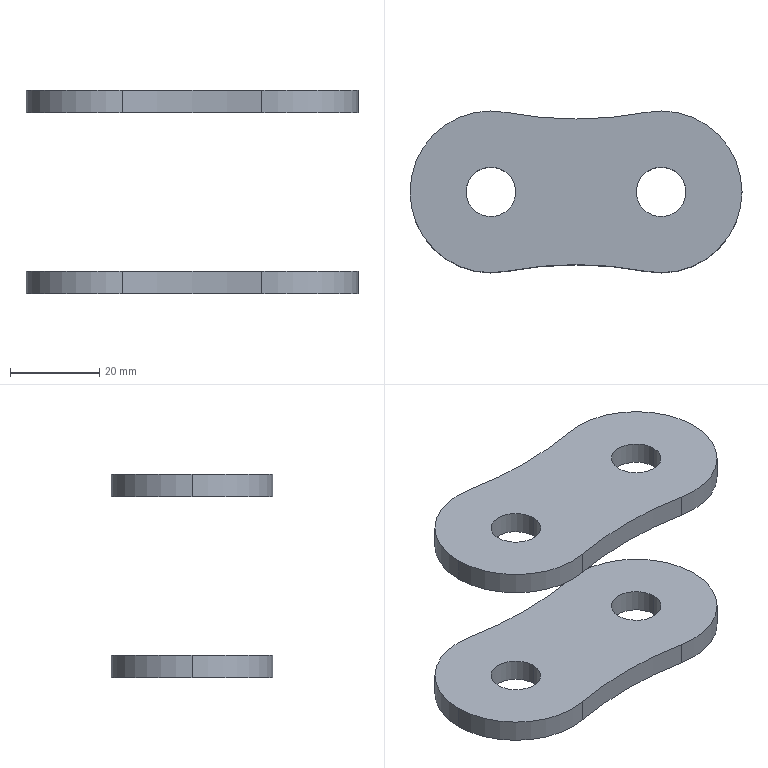Part | SolidWorks | features BaseBody 2 | 2 solids | 22 faces | box 74.3 x 36.2 x 45.44 mm | volume 21265 mm3 | cylinder 18 | plane 4 | commonest cylinder face diameters 11.11 x8 36.2 x6 166.109 x4
STEP:
#1=CARTESIAN_POINT('',(-24.605,0.,22.72));
#2=VERTEX_POINT('',#1);
#3=CARTESIAN_POINT('',(-13.495,0.,22.72));
#4=VERTEX_POINT('',#3);
#5=CARTESIAN_POINT('',(-19.05,0.,22.72));
#6=DIRECTION('',(0.,0.,1.));
#7=DIRECTION('',(1.,0.,0.));
#8=AXIS2_PLACEMENT_3D('',#5,#6,#7);
#9=CIRCLE('',#8,5.555);
#10=EDGE_CURVE('',#2,#4,#9,.T.);
#11=ORIENTED_EDGE('',*,*,#10,.T.);
#12=CARTESIAN_POINT('',(-13.495,0.,17.73));
#13=VERTEX_POINT('',#12);
#14=CARTESIAN_POINT('',(-13.495,0.,22.72));
#15=DIRECTION('',(0.,0.,-1.));
#16=VECTOR('',#15,1000.);
#17=LINE('',#14,#16);
#18=EDGE_CURVE('',#4,#13,#17,.T.);
#19=ORIENTED_EDGE('',*,*,#18,.T.);
#20=CARTESIAN_POINT('',(-24.605,0.,17.73));
#21=VERTEX_POINT('',#20);
#22=CARTESIAN_POINT('',(-19.05,0.,17.73));
#23=DIRECTION('',(0.,0.,1.));
#24=DIRECTION('',(1.,0.,0.));
#25=AXIS2_PLACEMENT_3D('',#22,#23,#24);
#26=CIRCLE('',#25,5.555);
#27=EDGE_CURVE('',#21,#13,#26,.T.);
#28=ORIENTED_EDGE('',*,*,#27,.F.);
#29=CARTESIAN_POINT('',(-24.605,0.,22.72));
#30=DIRECTION('',(0.,0.,-1.));
#31=VECTOR('',#30,1000.);
#32=LINE('',#29,#31);
#33=EDGE_CURVE('',#2,#21,#32,.T.);
#34=ORIENTED_EDGE('',*,*,#33,.F.);
#35=EDGE_LOOP('',(#11,#19,#28,#34));
#36=FACE_OUTER_BOUND('',#35,.T.);
#37=CARTESIAN_POINT('',(-19.05,0.,22.72));
#38=DIRECTION('',(0.,0.,-1.));
#39=DIRECTION('',(-1.,0.,0.));
#40=AXIS2_PLACEMENT_3D('',#37,#38,#39);
#41=CYLINDRICAL_SURFACE('',#40,5.555);
#42=ADVANCED_FACE('',(#36),#41,.F.);
#43=CARTESIAN_POINT('',(13.495,0.,22.72));
#44=VERTEX_POINT('',#43);
#45=CARTESIAN_POINT('',(24.605,0.,22.72));
#46=VERTEX_POINT('',#45);
#47=CARTESIAN_POINT('',(19.05,0.,22.72));
#48=DIRECTION('',(0.,0.,1.));
#49=DIRECTION('',(1.,0.,0.));
#50=AXIS2_PLACEMENT_3D('',#47,#48,#49);
#51=CIRCLE('',#50,5.555);
#52=EDGE_CURVE('',#44,#46,#51,.T.);
#53=ORIENTED_EDGE('',*,*,#52,.T.);
#54=CARTESIAN_POINT('',(24.605,0.,17.73));
#55=VERTEX_POINT('',#54);
#56=CARTESIAN_POINT('',(24.605,0.,22.72));
#57=DIRECTION('',(0.,0.,-1.));
#58=VECTOR('',#57,1000.);
#59=LINE('',#56,#58);
#60=EDGE_CURVE('',#46,#55,#59,.T.);
#61=ORIENTED_EDGE('',*,*,#60,.T.);
#62=CARTESIAN_POINT('',(13.495,0.,17.73));
#63=VERTEX_POINT('',#62);
#64=CARTESIAN_POINT('',(19.05,0.,17.73));
#65=DIRECTION('',(0.,0.,1.));
#66=DIRECTION('',(1.,0.,0.));
#67=AXIS2_PLACEMENT_3D('',#64,#65,#66);
#68=CIRCLE('',#67,5.555);
#69=EDGE_CURVE('',#63,#55,#68,.T.);
#70=ORIENTED_EDGE('',*,*,#69,.F.);
#71=CARTESIAN_POINT('',(13.495,0.,22.72));
#72=DIRECTION('',(0.,0.,-1.));
#73=VECTOR('',#72,1000.);
#74=LINE('',#71,#73);
#75=EDGE_CURVE('',#44,#63,#74,.T.);
#76=ORIENTED_EDGE('',*,*,#75,.F.);
#77=EDGE_LOOP('',(#53,#61,#70,#76));
#78=FACE_OUTER_BOUND('',#77,.T.);
#79=CARTESIAN_POINT('',(19.05,0.,22.72));
#80=DIRECTION('',(0.,0.,-1.));
#81=DIRECTION('',(-1.,0.,0.));
#82=AXIS2_PLACEMENT_3D('',#79,#80,#81);
#83=CYLINDRICAL_SURFACE('',#82,5.555);
#84=ADVANCED_FACE('',(#78),#83,.F.);
#85=CARTESIAN_POINT('',(-37.15,0.,22.72));
#86=VERTEX_POINT('',#85);
#87=CARTESIAN_POINT('',(-15.641,-17.776,22.72));
#88=VERTEX_POINT('',#87);
#89=CARTESIAN_POINT('',(-19.05,0.,22.72));
#90=DIRECTION('',(0.,0.,1.));
#91=DIRECTION('',(1.,0.,0.));
#92=AXIS2_PLACEMENT_3D('',#89,#90,#91);
#93=CIRCLE('',#92,18.1);
#94=EDGE_CURVE('',#86,#88,#93,.T.);
#95=ORIENTED_EDGE('',*,*,#94,.F.);
#96=CARTESIAN_POINT('',(-37.15,0.,17.73));
#97=VERTEX_POINT('',#96);
#98=CARTESIAN_POINT('',(-37.15,0.,22.72));
#99=DIRECTION('',(0.,0.,-1.));
#100=VECTOR('',#99,1000.);
#101=LINE('',#98,#100);
#102=EDGE_CURVE('',#86,#97,#101,.T.);
#103=ORIENTED_EDGE('',*,*,#102,.T.);
#104=CARTESIAN_POINT('',(-15.641,-17.776,17.73));
#105=VERTEX_POINT('',#104);
#106=CARTESIAN_POINT('',(-19.05,0.,17.73));
#107=DIRECTION('',(0.,0.,1.));
#108=DIRECTION('',(1.,0.,0.));
#109=AXIS2_PLACEMENT_3D('',#106,#107,#108);
#110=CIRCLE('',#109,18.1);
#111=EDGE_CURVE('',#97,#105,#110,.T.);
#112=ORIENTED_EDGE('',*,*,#111,.T.);
#113=CARTESIAN_POINT('',(-15.641,-17.776,22.72));
#114=DIRECTION('',(0.,0.,-1.));
#115=VECTOR('',#114,1000.);
#116=LINE('',#113,#115);
#117=EDGE_CURVE('',#88,#105,#116,.T.);
#118=ORIENTED_EDGE('',*,*,#117,.F.);
#119=EDGE_LOOP('',(#95,#103,#112,#118));
#120=FACE_OUTER_BOUND('',#119,.T.);
#121=CARTESIAN_POINT('',(-19.05,0.,22.72));
#122=DIRECTION('',(0.,0.,-1.));
#123=DIRECTION('',(-1.,0.,0.));
#124=AXIS2_PLACEMENT_3D('',#121,#122,#123);
#125=CYLINDRICAL_SURFACE('',#124,18.1);
#126=ADVANCED_FACE('',(#120),#125,.T.);
#127=ORIENTED_EDGE('',*,*,#52,.F.);
#128=CARTESIAN_POINT('',(19.05,0.,22.72));
#129=DIRECTION('',(0.,0.,1.));
#130=DIRECTION('',(1.,0.,0.));
#131=AXIS2_PLACEMENT_3D('',#128,#129,#130);
#132=CIRCLE('',#131,5.555);
#133=EDGE_CURVE('',#46,#44,#132,.T.);
#134=ORIENTED_EDGE('',*,*,#133,.F.);
#135=EDGE_LOOP('',(#127,#134));
#136=FACE_BOUND('',#135,.T.);
#137=CARTESIAN_POINT('',(15.641,-17.776,22.72));
#138=VERTEX_POINT('',#137);
#139=CARTESIAN_POINT('',(0.,-99.344,22.72));
#140=DIRECTION('',(0.,0.,-1.));
#141=DIRECTION('',(1.,0.,0.));
#142=AXIS2_PLACEMENT_3D('',#139,#140,#141);
#143=CIRCLE('',#142,83.054);
#144=EDGE_CURVE('',#88,#138,#143,.T.);
#145=ORIENTED_EDGE('',*,*,#144,.T.);
#146=CARTESIAN_POINT('',(15.641,17.776,22.72));
#147=VERTEX_POINT('',#146);
#148=CARTESIAN_POINT('',(19.05,0.,22.72));
#149=DIRECTION('',(0.,0.,1.));
#150=DIRECTION('',(1.,0.,0.));
#151=AXIS2_PLACEMENT_3D('',#148,#149,#150);
#152=CIRCLE('',#151,18.1);
#153=EDGE_CURVE('',#138,#147,#152,.T.);
#154=ORIENTED_EDGE('',*,*,#153,.T.);
#155=CARTESIAN_POINT('',(-15.641,17.776,22.72));
#156=VERTEX_POINT('',#155);
#157=CARTESIAN_POINT('',(0.,99.344,22.72));
#158=DIRECTION('',(0.,0.,-1.));
#159=DIRECTION('',(-1.,0.,0.));
#160=AXIS2_PLACEMENT_3D('',#157,#158,#159);
#161=CIRCLE('',#160,83.054);
#162=EDGE_CURVE('',#147,#156,#161,.T.);
#163=ORIENTED_EDGE('',*,*,#162,.T.);
#164=CARTESIAN_POINT('',(-19.05,0.,22.72));
#165=DIRECTION('',(0.,0.,1.));
#166=DIRECTION('',(1.,0.,0.));
#167=AXIS2_PLACEMENT_3D('',#164,#165,#166);
#168=CIRCLE('',#167,18.1);
#169=EDGE_CURVE('',#156,#86,#168,.T.);
#170=ORIENTED_EDGE('',*,*,#169,.T.);
#171=ORIENTED_EDGE('',*,*,#94,.T.);
#172=EDGE_LOOP('',(#145,#154,#163,#170,#171));
#173=FACE_OUTER_BOUND('',#172,.T.);
#174=ORIENTED_EDGE('',*,*,#10,.F.);
#175=CARTESIAN_POINT('',(-19.05,0.,22.72));
#176=DIRECTION('',(0.,0.,1.));
#177=DIRECTION('',(1.,0.,0.));
#178=AXIS2_PLACEMENT_3D('',#175,#176,#177);
#179=CIRCLE('',#178,5.555);
#180=EDGE_CURVE('',#4,#2,#179,.T.);
#181=ORIENTED_EDGE('',*,*,#180,.F.);
#182=EDGE_LOOP('',(#174,#181));
#183=FACE_BOUND('',#182,.T.);
#184=CARTESIAN_POINT('',(-9.525,-49.672,22.72));
#185=DIRECTION('',(0.,0.,1.));
#186=DIRECTION('',(1.,0.,0.));
#187=AXIS2_PLACEMENT_3D('',#184,#185,#186);
#188=PLANE('',#187);
#189=ADVANCED_FACE('',(#136,#173,#183),#188,.T.);
#190=CARTESIAN_POINT('',(15.641,-17.776,17.73));
#191=VERTEX_POINT('',#190);
#192=CARTESIAN_POINT('',(0.,-99.344,17.73));
#193=DIRECTION('',(0.,0.,-1.));
#194=DIRECTION('',(1.,0.,0.));
#195=AXIS2_PLACEMENT_3D('',#192,#193,#194);
#196=CIRCLE('',#195,83.054);
#197=EDGE_CURVE('',#105,#191,#196,.T.);
#198=ORIENTED_EDGE('',*,*,#197,.F.);
#199=ORIENTED_EDGE('',*,*,#111,.F.);
#200=CARTESIAN_POINT('',(-15.641,17.776,17.73));
#201=VERTEX_POINT('',#200);
#202=CARTESIAN_POINT('',(-19.05,0.,17.73));
#203=DIRECTION('',(0.,0.,1.));
#204=DIRECTION('',(1.,0.,0.));
#205=AXIS2_PLACEMENT_3D('',#202,#203,#204);
#206=CIRCLE('',#205,18.1);
#207=EDGE_CURVE('',#201,#97,#206,.T.);
#208=ORIENTED_EDGE('',*,*,#207,.F.);
#209=CARTESIAN_POINT('',(15.641,17.776,17.73));
#210=VERTEX_POINT('',#209);
#211=CARTESIAN_POINT('',(0.,99.344,17.73));
#212=DIRECTION('',(0.,0.,-1.));
#213=DIRECTION('',(-1.,0.,0.));
#214=AXIS2_PLACEMENT_3D('',#211,#212,#213);
#215=CIRCLE('',#214,83.054);
#216=EDGE_CURVE('',#210,#201,#215,.T.);
#217=ORIENTED_EDGE('',*,*,#216,.F.);
#218=CARTESIAN_POINT('',(19.05,0.,17.73));
#219=DIRECTION('',(0.,0.,1.));
#220=DIRECTION('',(1.,0.,0.));
#221=AXIS2_PLACEMENT_3D('',#218,#219,#220);
#222=CIRCLE('',#221,18.1);
#223=EDGE_CURVE('',#191,#210,#222,.T.);
#224=ORIENTED_EDGE('',*,*,#223,.F.);
#225=EDGE_LOOP('',(#198,#199,#208,#217,#224));
#226=FACE_OUTER_BOUND('',#225,.T.);
#227=ORIENTED_EDGE('',*,*,#69,.T.);
#228=CARTESIAN_POINT('',(19.05,0.,17.73));
#229=DIRECTION('',(0.,0.,1.));
#230=DIRECTION('',(1.,0.,0.));
#231=AXIS2_PLACEMENT_3D('',#228,#229,#230);
#232=CIRCLE('',#231,5.555);
#233=EDGE_CURVE('',#55,#63,#232,.T.);
#234=ORIENTED_EDGE('',*,*,#233,.T.);
#235=EDGE_LOOP('',(#227,#234));
#236=FACE_BOUND('',#235,.T.);
#237=ORIENTED_EDGE('',*,*,#27,.T.);
#238=CARTESIAN_POINT('',(-19.05,0.,17.73));
#239=DIRECTION('',(0.,0.,1.));
#240=DIRECTION('',(1.,0.,0.));
#241=AXIS2_PLACEMENT_3D('',#238,#239,#240);
#242=CIRCLE('',#241,5.555);
#243=EDGE_CURVE('',#13,#21,#242,.T.);
#244=ORIENTED_EDGE('',*,*,#243,.T.);
#245=EDGE_LOOP('',(#237,#244));
#246=FACE_BOUND('',#245,.T.);
#247=CARTESIAN_POINT('',(-9.525,-49.672,17.73));
#248=DIRECTION('',(0.,0.,1.));
#249=DIRECTION('',(1.,0.,0.));
#250=AXIS2_PLACEMENT_3D('',#247,#248,#249);
#251=PLANE('',#250);
#252=ADVANCED_FACE('',(#226,#236,#246),#251,.F.);
#253=ORIENTED_EDGE('',*,*,#197,.T.);
#254=CARTESIAN_POINT('',(15.641,-17.776,22.72));
#255=DIRECTION('',(0.,0.,-1.));
#256=VECTOR('',#255,1000.);
#257=LINE('',#254,#256);
#258=EDGE_CURVE('',#138,#191,#257,.T.);
#259=ORIENTED_EDGE('',*,*,#258,.F.);
#260=ORIENTED_EDGE('',*,*,#144,.F.);
#261=ORIENTED_EDGE('',*,*,#117,.T.);
#262=EDGE_LOOP('',(#253,#259,#260,#261));
#263=FACE_OUTER_BOUND('',#262,.T.);
#264=CARTESIAN_POINT('',(0.,-99.344,22.72));
#265=DIRECTION('',(0.,0.,-1.));
#266=DIRECTION('',(-1.,0.,0.));
#267=AXIS2_PLACEMENT_3D('',#264,#265,#266);
#268=CYLINDRICAL_SURFACE('',#267,83.054);
#269=ADVANCED_FACE('',(#263),#268,.F.);
#270=ORIENTED_EDGE('',*,*,#223,.T.);
#271=CARTESIAN_POINT('',(15.641,17.776,22.72));
#272=DIRECTION('',(0.,0.,-1.));
#273=VECTOR('',#272,1000.);
#274=LINE('',#271,#273);
#275=EDGE_CURVE('',#147,#210,#274,.T.);
#276=ORIENTED_EDGE('',*,*,#275,.F.);
#277=ORIENTED_EDGE('',*,*,#153,.F.);
#278=ORIENTED_EDGE('',*,*,#258,.T.);
#279=EDGE_LOOP('',(#270,#276,#277,#278));
#280=FACE_OUTER_BOUND('',#279,.T.);
#281=CARTESIAN_POINT('',(19.05,0.,22.72));
#282=DIRECTION('',(0.,0.,-1.));
#283=DIRECTION('',(-1.,0.,0.));
#284=AXIS2_PLACEMENT_3D('',#281,#282,#283);
#285=CYLINDRICAL_SURFACE('',#284,18.1);
#286=ADVANCED_FACE('',(#280),#285,.T.);
#287=ORIENTED_EDGE('',*,*,#216,.T.);
#288=CARTESIAN_POINT('',(-15.641,17.776,22.72));
#289=DIRECTION('',(0.,0.,-1.));
#290=VECTOR('',#289,1000.);
#291=LINE('',#288,#290);
#292=EDGE_CURVE('',#156,#201,#291,.T.);
#293=ORIENTED_EDGE('',*,*,#292,.F.);
#294=ORIENTED_EDGE('',*,*,#162,.F.);
#295=ORIENTED_EDGE('',*,*,#275,.T.);
#296=EDGE_LOOP('',(#287,#293,#294,#295));
#297=FACE_OUTER_BOUND('',#296,.T.);
#298=CARTESIAN_POINT('',(0.,99.344,22.72));
#299=DIRECTION('',(0.,0.,-1.));
#300=DIRECTION('',(-1.,0.,0.));
#301=AXIS2_PLACEMENT_3D('',#298,#299,#300);
#302=CYLINDRICAL_SURFACE('',#301,83.054);
#303=ADVANCED_FACE('',(#297),#302,.F.);
#304=ORIENTED_EDGE('',*,*,#102,.F.);
#305=ORIENTED_EDGE('',*,*,#169,.F.);
#306=ORIENTED_EDGE('',*,*,#292,.T.);
#307=ORIENTED_EDGE('',*,*,#207,.T.);
#308=EDGE_LOOP('',(#304,#305,#306,#307));
#309=FACE_OUTER_BOUND('',#308,.T.);
#310=CARTESIAN_POINT('',(-19.05,0.,22.72));
#311=DIRECTION('',(0.,0.,-1.));
#312=DIRECTION('',(-1.,0.,0.));
#313=AXIS2_PLACEMENT_3D('',#310,#311,#312);
#314=CYLINDRICAL_SURFACE('',#313,18.1);
#315=ADVANCED_FACE('',(#309),#314,.T.);
#316=ORIENTED_EDGE('',*,*,#60,.F.);
#317=ORIENTED_EDGE('',*,*,#133,.T.);
#318=ORIENTED_EDGE('',*,*,#75,.T.);
#319=ORIENTED_EDGE('',*,*,#233,.F.);
#320=EDGE_LOOP('',(#316,#317,#318,#319));
#321=FACE_OUTER_BOUND('',#320,.T.);
#322=CARTESIAN_POINT('',(19.05,0.,22.72));
#323=DIRECTION('',(0.,0.,-1.));
#324=DIRECTION('',(-1.,0.,0.));
#325=AXIS2_PLACEMENT_3D('',#322,#323,#324);
#326=CYLINDRICAL_SURFACE('',#325,5.555);
#327=ADVANCED_FACE('',(#321),#326,.F.);
#328=ORIENTED_EDGE('',*,*,#18,.F.);
#329=ORIENTED_EDGE('',*,*,#180,.T.);
#330=ORIENTED_EDGE('',*,*,#33,.T.);
#331=ORIENTED_EDGE('',*,*,#243,.F.);
#332=EDGE_LOOP('',(#328,#329,#330,#331));
#333=FACE_OUTER_BOUND('',#332,.T.);
#334=CARTESIAN_POINT('',(-19.05,0.,22.72));
#335=DIRECTION('',(0.,0.,-1.));
#336=DIRECTION('',(-1.,0.,0.));
#337=AXIS2_PLACEMENT_3D('',#334,#335,#336);
#338=CYLINDRICAL_SURFACE('',#337,5.555);
#339=ADVANCED_FACE('',(#333),#338,.F.);
#340=CLOSED_SHELL('',(#42,#84,#126,#189,#252,#269,#286,#303,#315,#327,#339));
#341=MANIFOLD_SOLID_BREP('',#340);
#342=CARTESIAN_POINT('',(-13.495,0.,-22.72));
#343=VERTEX_POINT('',#342);
#344=CARTESIAN_POINT('',(-24.605,0.,-22.72));
#345=VERTEX_POINT('',#344);
#346=CARTESIAN_POINT('',(-19.05,0.,-22.72));
#347=DIRECTION('',(0.,0.,1.));
#348=DIRECTION('',(1.,0.,0.));
#349=AXIS2_PLACEMENT_3D('',#346,#347,#348);
#350=CIRCLE('',#349,5.555);
#351=EDGE_CURVE('',#343,#345,#350,.T.);
#352=ORIENTED_EDGE('',*,*,#351,.F.);
#353=CARTESIAN_POINT('',(-13.495,0.,-17.73));
#354=VERTEX_POINT('',#353);
#355=CARTESIAN_POINT('',(-13.495,0.,-22.72));
#356=DIRECTION('',(0.,0.,1.));
#357=VECTOR('',#356,1000.);
#358=LINE('',#355,#357);
#359=EDGE_CURVE('',#343,#354,#358,.T.);
#360=ORIENTED_EDGE('',*,*,#359,.T.);
#361=CARTESIAN_POINT('',(-24.605,0.,-17.73));
#362=VERTEX_POINT('',#361);
#363=CARTESIAN_POINT('',(-19.05,0.,-17.73));
#364=DIRECTION('',(0.,0.,1.));
#365=DIRECTION('',(1.,0.,0.));
#366=AXIS2_PLACEMENT_3D('',#363,#364,#365);
#367=CIRCLE('',#366,5.555);
#368=EDGE_CURVE('',#354,#362,#367,.T.);
#369=ORIENTED_EDGE('',*,*,#368,.T.);
#370=CARTESIAN_POINT('',(-24.605,0.,-22.72));
#371=DIRECTION('',(0.,0.,1.));
#372=VECTOR('',#371,1000.);
#373=LINE('',#370,#372);
#374=EDGE_CURVE('',#345,#362,#373,.T.);
#375=ORIENTED_EDGE('',*,*,#374,.F.);
#376=EDGE_LOOP('',(#352,#360,#369,#375));
#377=FACE_OUTER_BOUND('',#376,.T.);
#378=CARTESIAN_POINT('',(-19.05,0.,-22.72));
#379=DIRECTION('',(0.,0.,1.));
#380=DIRECTION('',(-1.,0.,0.));
#381=AXIS2_PLACEMENT_3D('',#378,#379,#380);
#382=CYLINDRICAL_SURFACE('',#381,5.555);
#383=ADVANCED_FACE('',(#377),#382,.F.);
#384=CARTESIAN_POINT('',(24.605,0.,-22.72));
#385=VERTEX_POINT('',#384);
#386=CARTESIAN_POINT('',(13.495,0.,-22.72));
#387=VERTEX_POINT('',#386);
#388=CARTESIAN_POINT('',(19.05,0.,-22.72));
#389=DIRECTION('',(0.,0.,1.));
#390=DIRECTION('',(1.,0.,0.));
#391=AXIS2_PLACEMENT_3D('',#388,#389,#390);
#392=CIRCLE('',#391,5.555);
#393=EDGE_CURVE('',#385,#387,#392,.T.);
#394=ORIENTED_EDGE('',*,*,#393,.F.);
#395=CARTESIAN_POINT('',(24.605,0.,-17.73));
#396=VERTEX_POINT('',#395);
#397=CARTESIAN_POINT('',(24.605,0.,-22.72));
#398=DIRECTION('',(0.,0.,1.));
#399=VECTOR('',#398,1000.);
#400=LINE('',#397,#399);
#401=EDGE_CURVE('',#385,#396,#400,.T.);
#402=ORIENTED_EDGE('',*,*,#401,.T.);
#403=CARTESIAN_POINT('',(13.495,0.,-17.73));
#404=VERTEX_POINT('',#403);
#405=CARTESIAN_POINT('',(19.05,0.,-17.73));
#406=DIRECTION('',(0.,0.,1.));
#407=DIRECTION('',(1.,0.,0.));
#408=AXIS2_PLACEMENT_3D('',#405,#406,#407);
#409=CIRCLE('',#408,5.555);
#410=EDGE_CURVE('',#396,#404,#409,.T.);
#411=ORIENTED_EDGE('',*,*,#410,.T.);
#412=CARTESIAN_POINT('',(13.495,0.,-22.72));
#413=DIRECTION('',(0.,0.,1.));
#414=VECTOR('',#413,1000.);
#415=LINE('',#412,#414);
#416=EDGE_CURVE('',#387,#404,#415,.T.);
#417=ORIENTED_EDGE('',*,*,#416,.F.);
#418=EDGE_LOOP('',(#394,#402,#411,#417));
#419=FACE_OUTER_BOUND('',#418,.T.);
#420=CARTESIAN_POINT('',(19.05,0.,-22.72));
#421=DIRECTION('',(0.,0.,1.));
#422=DIRECTION('',(-1.,0.,0.));
#423=AXIS2_PLACEMENT_3D('',#420,#421,#422);
#424=CYLINDRICAL_SURFACE('',#423,5.555);
#425=ADVANCED_FACE('',(#419),#424,.F.);
#426=CARTESIAN_POINT('',(-15.641,17.776,-22.72));
#427=VERTEX_POINT('',#426);
#428=CARTESIAN_POINT('',(-37.15,0.,-22.72));
#429=VERTEX_POINT('',#428);
#430=CARTESIAN_POINT('',(-19.05,0.,-22.72));
#431=DIRECTION('',(0.,0.,1.));
#432=DIRECTION('',(1.,0.,0.));
#433=AXIS2_PLACEMENT_3D('',#430,#431,#432);
#434=CIRCLE('',#433,18.1);
#435=EDGE_CURVE('',#427,#429,#434,.T.);
#436=ORIENTED_EDGE('',*,*,#435,.T.);
#437=CARTESIAN_POINT('',(-37.15,0.,-17.73));
#438=VERTEX_POINT('',#437);
#439=CARTESIAN_POINT('',(-37.15,0.,-22.72));
#440=DIRECTION('',(0.,0.,1.));
#441=VECTOR('',#440,1000.);
#442=LINE('',#439,#441);
#443=EDGE_CURVE('',#429,#438,#442,.T.);
#444=ORIENTED_EDGE('',*,*,#443,.T.);
#445=CARTESIAN_POINT('',(-15.641,17.776,-17.73));
#446=VERTEX_POINT('',#445);
#447=CARTESIAN_POINT('',(-19.05,0.,-17.73));
#448=DIRECTION('',(0.,0.,1.));
#449=DIRECTION('',(1.,0.,0.));
#450=AXIS2_PLACEMENT_3D('',#447,#448,#449);
#451=CIRCLE('',#450,18.1);
#452=EDGE_CURVE('',#446,#438,#451,.T.);
#453=ORIENTED_EDGE('',*,*,#452,.F.);
#454=CARTESIAN_POINT('',(-15.641,17.776,-22.72));
#455=DIRECTION('',(0.,0.,1.));
#456=VECTOR('',#455,1000.);
#457=LINE('',#454,#456);
#458=EDGE_CURVE('',#427,#446,#457,.T.);
#459=ORIENTED_EDGE('',*,*,#458,.F.);
#460=EDGE_LOOP('',(#436,#444,#453,#459));
#461=FACE_OUTER_BOUND('',#460,.T.);
#462=CARTESIAN_POINT('',(-19.05,0.,-22.72));
#463=DIRECTION('',(0.,0.,1.));
#464=DIRECTION('',(-1.,0.,0.));
#465=AXIS2_PLACEMENT_3D('',#462,#463,#464);
#466=CYLINDRICAL_SURFACE('',#465,18.1);
#467=ADVANCED_FACE('',(#461),#466,.T.);
#468=CARTESIAN_POINT('',(19.05,0.,-22.72));
#469=DIRECTION('',(0.,0.,1.));
#470=DIRECTION('',(1.,0.,0.));
#471=AXIS2_PLACEMENT_3D('',#468,#469,#470);
#472=CIRCLE('',#471,5.555);
#473=EDGE_CURVE('',#387,#385,#472,.T.);
#474=ORIENTED_EDGE('',*,*,#473,.T.);
#475=ORIENTED_EDGE('',*,*,#393,.T.);
#476=EDGE_LOOP('',(#474,#475));
#477=FACE_BOUND('',#476,.T.);
#478=CARTESIAN_POINT('',(-15.641,-17.776,-22.72));
#479=VERTEX_POINT('',#478);
#480=CARTESIAN_POINT('',(15.641,-17.776,-22.72));
#481=VERTEX_POINT('',#480);
#482=CARTESIAN_POINT('',(0.,-99.344,-22.72));
#483=DIRECTION('',(0.,0.,-1.));
#484=DIRECTION('',(1.,0.,0.));
#485=AXIS2_PLACEMENT_3D('',#482,#483,#484);
#486=CIRCLE('',#485,83.054);
#487=EDGE_CURVE('',#479,#481,#486,.T.);
#488=ORIENTED_EDGE('',*,*,#487,.F.);
#489=CARTESIAN_POINT('',(-19.05,0.,-22.72));
#490=DIRECTION('',(0.,0.,1.));
#491=DIRECTION('',(1.,0.,0.));
#492=AXIS2_PLACEMENT_3D('',#489,#490,#491);
#493=CIRCLE('',#492,18.1);
#494=EDGE_CURVE('',#429,#479,#493,.T.);
#495=ORIENTED_EDGE('',*,*,#494,.F.);
#496=ORIENTED_EDGE('',*,*,#435,.F.);
#497=CARTESIAN_POINT('',(15.641,17.776,-22.72));
#498=VERTEX_POINT('',#497);
#499=CARTESIAN_POINT('',(0.,99.344,-22.72));
#500=DIRECTION('',(0.,0.,-1.));
#501=DIRECTION('',(-1.,0.,0.));
#502=AXIS2_PLACEMENT_3D('',#499,#500,#501);
#503=CIRCLE('',#502,83.054);
#504=EDGE_CURVE('',#498,#427,#503,.T.);
#505=ORIENTED_EDGE('',*,*,#504,.F.);
#506=CARTESIAN_POINT('',(19.05,0.,-22.72));
#507=DIRECTION('',(0.,0.,1.));
#508=DIRECTION('',(1.,0.,0.));
#509=AXIS2_PLACEMENT_3D('',#506,#507,#508);
#510=CIRCLE('',#509,18.1);
#511=EDGE_CURVE('',#481,#498,#510,.T.);
#512=ORIENTED_EDGE('',*,*,#511,.F.);
#513=EDGE_LOOP('',(#488,#495,#496,#505,#512));
#514=FACE_OUTER_BOUND('',#513,.T.);
#515=CARTESIAN_POINT('',(-19.05,0.,-22.72));
#516=DIRECTION('',(0.,0.,1.));
#517=DIRECTION('',(1.,0.,0.));
#518=AXIS2_PLACEMENT_3D('',#515,#516,#517);
#519=CIRCLE('',#518,5.555);
#520=EDGE_CURVE('',#345,#343,#519,.T.);
#521=ORIENTED_EDGE('',*,*,#520,.T.);
#522=ORIENTED_EDGE('',*,*,#351,.T.);
#523=EDGE_LOOP('',(#521,#522));
#524=FACE_BOUND('',#523,.T.);
#525=CARTESIAN_POINT('',(-9.525,-49.672,-22.72));
#526=DIRECTION('',(0.,0.,-1.));
#527=DIRECTION('',(1.,0.,0.));
#528=AXIS2_PLACEMENT_3D('',#525,#526,#527);
#529=PLANE('',#528);
#530=ADVANCED_FACE('',(#477,#514,#524),#529,.T.);
#531=CARTESIAN_POINT('',(-15.641,-17.776,-17.73));
#532=VERTEX_POINT('',#531);
#533=CARTESIAN_POINT('',(15.641,-17.776,-17.73));
#534=VERTEX_POINT('',#533);
#535=CARTESIAN_POINT('',(0.,-99.344,-17.73));
#536=DIRECTION('',(0.,0.,-1.));
#537=DIRECTION('',(1.,0.,0.));
#538=AXIS2_PLACEMENT_3D('',#535,#536,#537);
#539=CIRCLE('',#538,83.054);
#540=EDGE_CURVE('',#532,#534,#539,.T.);
#541=ORIENTED_EDGE('',*,*,#540,.T.);
#542=CARTESIAN_POINT('',(15.641,17.776,-17.73));
#543=VERTEX_POINT('',#542);
#544=CARTESIAN_POINT('',(19.05,0.,-17.73));
#545=DIRECTION('',(0.,0.,1.));
#546=DIRECTION('',(1.,0.,0.));
#547=AXIS2_PLACEMENT_3D('',#544,#545,#546);
#548=CIRCLE('',#547,18.1);
#549=EDGE_CURVE('',#534,#543,#548,.T.);
#550=ORIENTED_EDGE('',*,*,#549,.T.);
#551=CARTESIAN_POINT('',(0.,99.344,-17.73));
#552=DIRECTION('',(0.,0.,-1.));
#553=DIRECTION('',(-1.,0.,0.));
#554=AXIS2_PLACEMENT_3D('',#551,#552,#553);
#555=CIRCLE('',#554,83.054);
#556=EDGE_CURVE('',#543,#446,#555,.T.);
#557=ORIENTED_EDGE('',*,*,#556,.T.);
#558=ORIENTED_EDGE('',*,*,#452,.T.);
#559=CARTESIAN_POINT('',(-19.05,0.,-17.73));
#560=DIRECTION('',(0.,0.,1.));
#561=DIRECTION('',(1.,0.,0.));
#562=AXIS2_PLACEMENT_3D('',#559,#560,#561);
#563=CIRCLE('',#562,18.1);
#564=EDGE_CURVE('',#438,#532,#563,.T.);
#565=ORIENTED_EDGE('',*,*,#564,.T.);
#566=EDGE_LOOP('',(#541,#550,#557,#558,#565));
#567=FACE_OUTER_BOUND('',#566,.T.);
#568=CARTESIAN_POINT('',(19.05,0.,-17.73));
#569=DIRECTION('',(0.,0.,1.));
#570=DIRECTION('',(1.,0.,0.));
#571=AXIS2_PLACEMENT_3D('',#568,#569,#570);
#572=CIRCLE('',#571,5.555);
#573=EDGE_CURVE('',#404,#396,#572,.T.);
#574=ORIENTED_EDGE('',*,*,#573,.F.);
#575=ORIENTED_EDGE('',*,*,#410,.F.);
#576=EDGE_LOOP('',(#574,#575));
#577=FACE_BOUND('',#576,.T.);
#578=CARTESIAN_POINT('',(-19.05,0.,-17.73));
#579=DIRECTION('',(0.,0.,1.));
#580=DIRECTION('',(1.,0.,0.));
#581=AXIS2_PLACEMENT_3D('',#578,#579,#580);
#582=CIRCLE('',#581,5.555);
#583=EDGE_CURVE('',#362,#354,#582,.T.);
#584=ORIENTED_EDGE('',*,*,#583,.F.);
#585=ORIENTED_EDGE('',*,*,#368,.F.);
#586=EDGE_LOOP('',(#584,#585));
#587=FACE_BOUND('',#586,.T.);
#588=CARTESIAN_POINT('',(-9.525,-49.672,-17.73));
#589=DIRECTION('',(0.,0.,-1.));
#590=DIRECTION('',(1.,0.,0.));
#591=AXIS2_PLACEMENT_3D('',#588,#589,#590);
#592=PLANE('',#591);
#593=ADVANCED_FACE('',(#567,#577,#587),#592,.F.);
#594=ORIENTED_EDGE('',*,*,#540,.F.);
#595=CARTESIAN_POINT('',(-15.641,-17.776,-22.72));
#596=DIRECTION('',(0.,0.,1.));
#597=VECTOR('',#596,1000.);
#598=LINE('',#595,#597);
#599=EDGE_CURVE('',#479,#532,#598,.T.);
#600=ORIENTED_EDGE('',*,*,#599,.F.);
#601=ORIENTED_EDGE('',*,*,#487,.T.);
#602=CARTESIAN_POINT('',(15.641,-17.776,-22.72));
#603=DIRECTION('',(0.,0.,1.));
#604=VECTOR('',#603,1000.);
#605=LINE('',#602,#604);
#606=EDGE_CURVE('',#481,#534,#605,.T.);
#607=ORIENTED_EDGE('',*,*,#606,.T.);
#608=EDGE_LOOP('',(#594,#600,#601,#607));
#609=FACE_OUTER_BOUND('',#608,.T.);
#610=CARTESIAN_POINT('',(0.,-99.344,-22.72));
#611=DIRECTION('',(0.,0.,1.));
#612=DIRECTION('',(-1.,0.,0.));
#613=AXIS2_PLACEMENT_3D('',#610,#611,#612);
#614=CYLINDRICAL_SURFACE('',#613,83.054);
#615=ADVANCED_FACE('',(#609),#614,.F.);
#616=ORIENTED_EDGE('',*,*,#549,.F.);
#617=ORIENTED_EDGE('',*,*,#606,.F.);
#618=ORIENTED_EDGE('',*,*,#511,.T.);
#619=CARTESIAN_POINT('',(15.641,17.776,-22.72));
#620=DIRECTION('',(0.,0.,1.));
#621=VECTOR('',#620,1000.);
#622=LINE('',#619,#621);
#623=EDGE_CURVE('',#498,#543,#622,.T.);
#624=ORIENTED_EDGE('',*,*,#623,.T.);
#625=EDGE_LOOP('',(#616,#617,#618,#624));
#626=FACE_OUTER_BOUND('',#625,.T.);
#627=CARTESIAN_POINT('',(19.05,0.,-22.72));
#628=DIRECTION('',(0.,0.,1.));
#629=DIRECTION('',(-1.,0.,0.));
#630=AXIS2_PLACEMENT_3D('',#627,#628,#629);
#631=CYLINDRICAL_SURFACE('',#630,18.1);
#632=ADVANCED_FACE('',(#626),#631,.T.);
#633=ORIENTED_EDGE('',*,*,#556,.F.);
#634=ORIENTED_EDGE('',*,*,#623,.F.);
#635=ORIENTED_EDGE('',*,*,#504,.T.);
#636=ORIENTED_EDGE('',*,*,#458,.T.);
#637=EDGE_LOOP('',(#633,#634,#635,#636));
#638=FACE_OUTER_BOUND('',#637,.T.);
#639=CARTESIAN_POINT('',(0.,99.344,-22.72));
#640=DIRECTION('',(0.,0.,1.));
#641=DIRECTION('',(-1.,0.,0.));
#642=AXIS2_PLACEMENT_3D('',#639,#640,#641);
#643=CYLINDRICAL_SURFACE('',#642,83.054);
#644=ADVANCED_FACE('',(#638),#643,.F.);
#645=ORIENTED_EDGE('',*,*,#443,.F.);
#646=ORIENTED_EDGE('',*,*,#494,.T.);
#647=ORIENTED_EDGE('',*,*,#599,.T.);
#648=ORIENTED_EDGE('',*,*,#564,.F.);
#649=EDGE_LOOP('',(#645,#646,#647,#648));
#650=FACE_OUTER_BOUND('',#649,.T.);
#651=CARTESIAN_POINT('',(-19.05,0.,-22.72));
#652=DIRECTION('',(0.,0.,1.));
#653=DIRECTION('',(-1.,0.,0.));
#654=AXIS2_PLACEMENT_3D('',#651,#652,#653);
#655=CYLINDRICAL_SURFACE('',#654,18.1);
#656=ADVANCED_FACE('',(#650),#655,.T.);
#657=ORIENTED_EDGE('',*,*,#401,.F.);
#658=ORIENTED_EDGE('',*,*,#473,.F.);
#659=ORIENTED_EDGE('',*,*,#416,.T.);
#660=ORIENTED_EDGE('',*,*,#573,.T.);
#661=EDGE_LOOP('',(#657,#658,#659,#660));
#662=FACE_OUTER_BOUND('',#661,.T.);
#663=CARTESIAN_POINT('',(19.05,0.,-22.72));
#664=DIRECTION('',(0.,0.,1.));
#665=DIRECTION('',(-1.,0.,0.));
#666=AXIS2_PLACEMENT_3D('',#663,#664,#665);
#667=CYLINDRICAL_SURFACE('',#666,5.555);
#668=ADVANCED_FACE('',(#662),#667,.F.);
#669=ORIENTED_EDGE('',*,*,#359,.F.);
#670=ORIENTED_EDGE('',*,*,#520,.F.);
#671=ORIENTED_EDGE('',*,*,#374,.T.);
#672=ORIENTED_EDGE('',*,*,#583,.T.);
#673=EDGE_LOOP('',(#669,#670,#671,#672));
#674=FACE_OUTER_BOUND('',#673,.T.);
#675=CARTESIAN_POINT('',(-19.05,0.,-22.72));
#676=DIRECTION('',(0.,0.,1.));
#677=DIRECTION('',(-1.,0.,0.));
#678=AXIS2_PLACEMENT_3D('',#675,#676,#677);
#679=CYLINDRICAL_SURFACE('',#678,5.555);
#680=ADVANCED_FACE('',(#674),#679,.F.);
#681=CLOSED_SHELL('',(#383,#425,#467,#530,#593,#615,#632,#644,#656,#668,#680));
#682=MANIFOLD_SOLID_BREP('',#681);
#683=CARTESIAN_POINT('',(0.,0.,0.));
#684=DIRECTION('',(0.,0.,1.));
#685=DIRECTION('',(1.,0.,0.));
#686=AXIS2_PLACEMENT_3D('',#683,#684,#685);
#687=(LENGTH_UNIT()NAMED_UNIT(*)SI_UNIT(.MILLI.,.METRE.));
#688=UNCERTAINTY_MEASURE_WITH_UNIT(LENGTH_MEASURE(0.00001),#687,'','');
#689=(NAMED_UNIT(*)PLANE_ANGLE_UNIT()SI_UNIT($,.RADIAN.));
#690=(NAMED_UNIT(*)SI_UNIT($,.STERADIAN.)SOLID_ANGLE_UNIT());
#691=(GEOMETRIC_REPRESENTATION_CONTEXT(3)GLOBAL_UNCERTAINTY_ASSIGNED_CONTEXT((#688))GLOBAL_UNIT_ASSIGNED_CONTEXT((#687,#689,#690))REPRESENTATION_CONTEXT('',''));
#692=ADVANCED_BREP_SHAPE_REPRESENTATION('',(#341,#682,#686),#691);